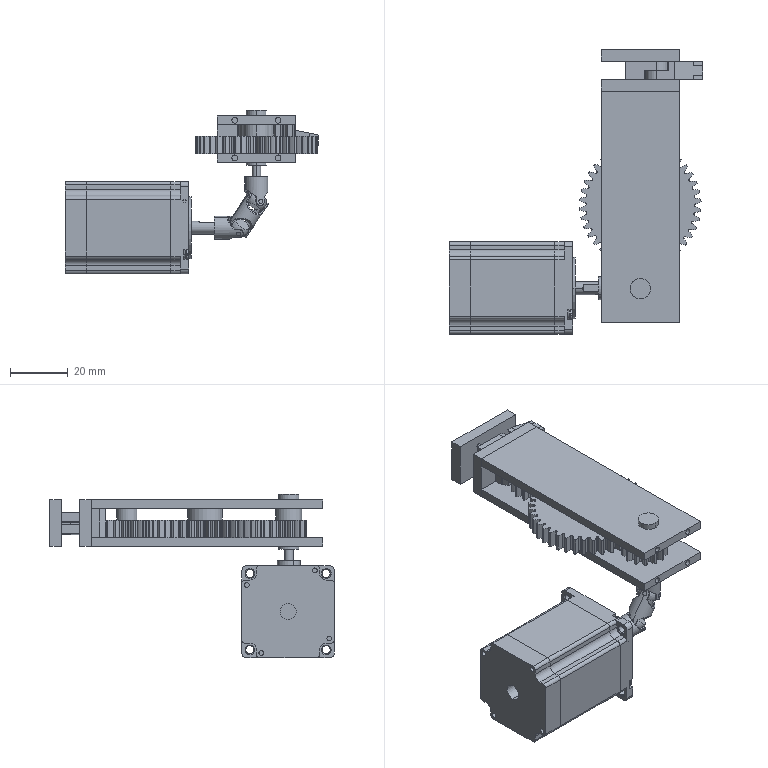Part | SolidWorks | features Cut 3, AEMSimFeature 1, InContextFeatHolder 1 | 36 solids | 1527 faces | box 87.535 x 98.347 x 56.623 mm | volume 68756 mm3 | cylinder 660 | plane 439 | torus 236 | sphere 154 | cone 38 | commonest cylinder face diameters 1.012 x80 16.21 x80 1.026 x56 6.947 x56 1.5 x52 42 x40